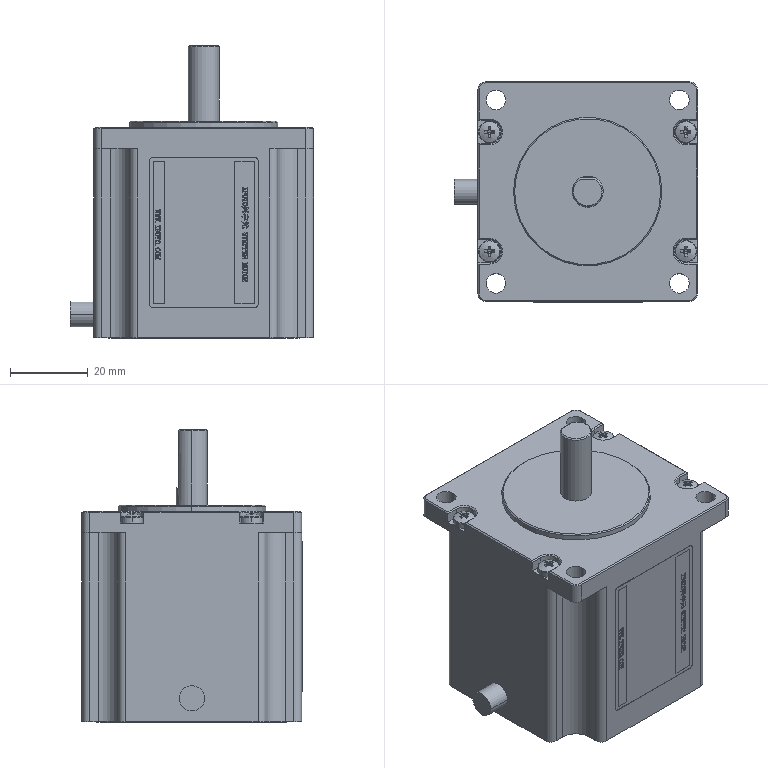Part | NX | features BREP 1 | 1 solid | 1847 faces | box 62.4 x 56.5 x 75.2 mm | volume 158259 mm3 | plane 1227 | spline 428 | cylinder 127 | cone 53 | torus 8 | sphere 4 | commonest cylinder face diameters 4 x12 2.5 x8 5 x8 5.6 x8 0.225 x6 6 x6